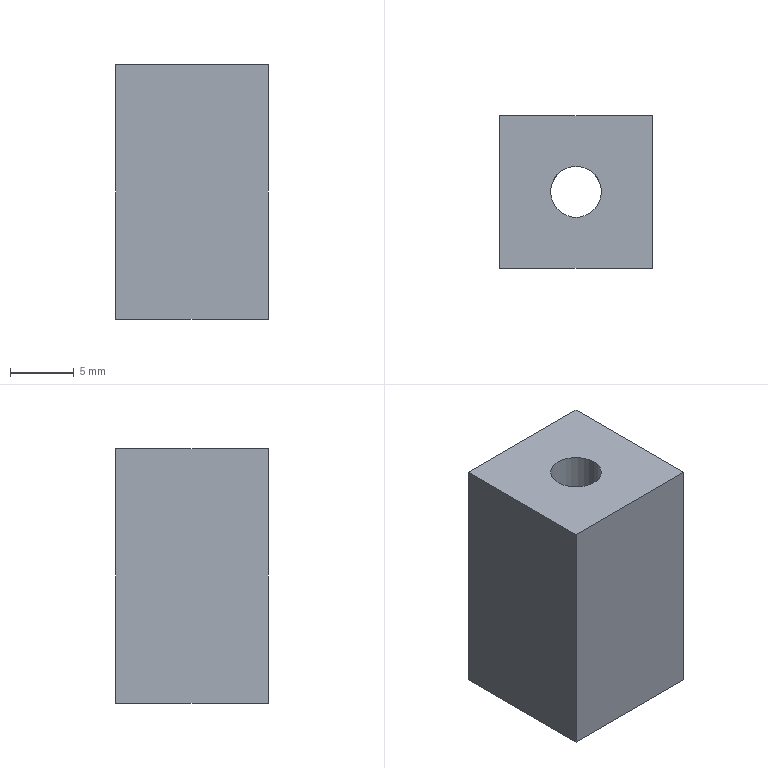Part | STEP file | Ngam kep 13 | 1 solid | 11 faces | box 12 x 12 x 20 mm | volume 2025 mm3 | plane 7 | cylinder 4 | commonest cylinder face diameters 4 x2 8 x2
STEP:
#1=CARTESIAN_POINT('',(0.,0.,0.));
#2=DIRECTION('',(0.,0.,1.));
#3=DIRECTION('',(1.,0.,0.));
#4=AXIS2_PLACEMENT_3D('',#1,#2,#3);
#5=CARTESIAN_POINT('',(-2.,0.,12.));
#6=VERTEX_POINT('',#5);
#7=CARTESIAN_POINT('',(-2.,0.,8.));
#8=VERTEX_POINT('',#7);
#9=CARTESIAN_POINT('',(-2.,0.,12.));
#10=DIRECTION('',(0.,0.,-1.));
#11=VECTOR('',#10,1.);
#12=LINE('',#9,#11);
#13=CARTESIAN_POINT('',(0.,0.,12.));
#14=DIRECTION('',(0.,0.,-1.));
#15=DIRECTION('',(-1.,0.,0.));
#16=AXIS2_PLACEMENT_3D('',#13,#14,#15);
#17=CYLINDRICAL_SURFACE('',#16,2.);
#18=CARTESIAN_POINT('',(6.283,0.));
#19=DIRECTION('',(0.,1.));
#20=VECTOR('',#19,1.);
#21=LINE('',#18,#20);
#22=(GEOMETRIC_REPRESENTATION_CONTEXT(2)PARAMETRIC_REPRESENTATION_CONTEXT()REPRESENTATION_CONTEXT('',''));
#23=DEFINITIONAL_REPRESENTATION('',(#21),#22);
#24=PCURVE('',#17,#23);
#25=CARTESIAN_POINT('',(0.,0.,12.));
#26=DIRECTION('',(0.,0.,-1.));
#27=DIRECTION('',(-1.,0.,0.));
#28=AXIS2_PLACEMENT_3D('',#25,#26,#27);
#29=CYLINDRICAL_SURFACE('',#28,2.);
#30=CARTESIAN_POINT('',(0.,0.));
#31=DIRECTION('',(0.,1.));
#32=VECTOR('',#31,1.);
#33=LINE('',#30,#32);
#34=(GEOMETRIC_REPRESENTATION_CONTEXT(2)PARAMETRIC_REPRESENTATION_CONTEXT()REPRESENTATION_CONTEXT('',''));
#35=DEFINITIONAL_REPRESENTATION('',(#33),#34);
#36=PCURVE('',#29,#35);
#37=SURFACE_CURVE('',#12,(#24,#36),.PCURVE_S1.);
#38=EDGE_CURVE('',#6,#8,#37,.T.);
#39=ORIENTED_EDGE('',*,*,#38,.T.);
#40=CARTESIAN_POINT('',(2.,0.,8.));
#41=VERTEX_POINT('',#40);
#42=CARTESIAN_POINT('',(0.,0.,8.));
#43=DIRECTION('',(0.,0.,1.));
#44=DIRECTION('',(1.,0.,0.));
#45=AXIS2_PLACEMENT_3D('',#42,#43,#44);
#46=CIRCLE('',#45,2.);
#47=CARTESIAN_POINT('',(9.425,4.));
#48=DIRECTION('',(-1.,0.));
#49=VECTOR('',#48,1.);
#50=LINE('',#47,#49);
#51=(GEOMETRIC_REPRESENTATION_CONTEXT(2)PARAMETRIC_REPRESENTATION_CONTEXT()REPRESENTATION_CONTEXT('',''));
#52=DEFINITIONAL_REPRESENTATION('',(#50),#51);
#53=PCURVE('',#17,#52);
#54=CARTESIAN_POINT('',(0.,0.,8.));
#55=DIRECTION('',(0.,0.,1.));
#56=DIRECTION('',(1.,0.,0.));
#57=AXIS2_PLACEMENT_3D('',#54,#55,#56);
#58=PLANE('',#57);
#59=CARTESIAN_POINT('',(0.,0.));
#60=DIRECTION('',(1.,0.));
#61=AXIS2_PLACEMENT_2D('',#59,#60);
#62=CIRCLE('',#61,2.);
#63=(GEOMETRIC_REPRESENTATION_CONTEXT(2)PARAMETRIC_REPRESENTATION_CONTEXT()REPRESENTATION_CONTEXT('',''));
#64=DEFINITIONAL_REPRESENTATION('',(#62),#63);
#65=PCURVE('',#58,#64);
#66=SURFACE_CURVE('',#46,(#53,#65),.PCURVE_S1.);
#67=EDGE_CURVE('',#8,#41,#66,.T.);
#68=ORIENTED_EDGE('',*,*,#67,.T.);
#69=CARTESIAN_POINT('',(2.,0.,12.));
#70=VERTEX_POINT('',#69);
#71=CARTESIAN_POINT('',(2.,0.,12.));
#72=DIRECTION('',(0.,0.,-1.));
#73=VECTOR('',#72,1.);
#74=LINE('',#71,#73);
#75=CARTESIAN_POINT('',(3.142,0.));
#76=DIRECTION('',(0.,1.));
#77=VECTOR('',#76,1.);
#78=LINE('',#75,#77);
#79=(GEOMETRIC_REPRESENTATION_CONTEXT(2)PARAMETRIC_REPRESENTATION_CONTEXT()REPRESENTATION_CONTEXT('',''));
#80=DEFINITIONAL_REPRESENTATION('',(#78),#79);
#81=PCURVE('',#17,#80);
#82=CARTESIAN_POINT('',(3.142,0.));
#83=DIRECTION('',(0.,1.));
#84=VECTOR('',#83,1.);
#85=LINE('',#82,#84);
#86=(GEOMETRIC_REPRESENTATION_CONTEXT(2)PARAMETRIC_REPRESENTATION_CONTEXT()REPRESENTATION_CONTEXT('',''));
#87=DEFINITIONAL_REPRESENTATION('',(#85),#86);
#88=PCURVE('',#29,#87);
#89=SURFACE_CURVE('',#74,(#81,#88),.PCURVE_S1.);
#90=EDGE_CURVE('',#70,#41,#89,.T.);
#91=ORIENTED_EDGE('',*,*,#90,.F.);
#92=CARTESIAN_POINT('',(0.,0.,12.));
#93=DIRECTION('',(0.,0.,1.));
#94=DIRECTION('',(1.,0.,0.));
#95=AXIS2_PLACEMENT_3D('',#92,#93,#94);
#96=CIRCLE('',#95,2.);
#97=CARTESIAN_POINT('',(9.425,0.));
#98=DIRECTION('',(-1.,0.));
#99=VECTOR('',#98,1.);
#100=LINE('',#97,#99);
#101=(GEOMETRIC_REPRESENTATION_CONTEXT(2)PARAMETRIC_REPRESENTATION_CONTEXT()REPRESENTATION_CONTEXT('',''));
#102=DEFINITIONAL_REPRESENTATION('',(#100),#101);
#103=PCURVE('',#17,#102);
#104=CARTESIAN_POINT('',(0.,0.,12.));
#105=DIRECTION('',(0.,0.,1.));
#106=DIRECTION('',(1.,0.,0.));
#107=AXIS2_PLACEMENT_3D('',#104,#105,#106);
#108=PLANE('',#107);
#109=CARTESIAN_POINT('',(0.,0.));
#110=DIRECTION('',(1.,0.));
#111=AXIS2_PLACEMENT_2D('',#109,#110);
#112=CIRCLE('',#111,2.);
#113=(GEOMETRIC_REPRESENTATION_CONTEXT(2)PARAMETRIC_REPRESENTATION_CONTEXT()REPRESENTATION_CONTEXT('',''));
#114=DEFINITIONAL_REPRESENTATION('',(#112),#113);
#115=PCURVE('',#108,#114);
#116=SURFACE_CURVE('',#96,(#103,#115),.PCURVE_S1.);
#117=EDGE_CURVE('',#6,#70,#116,.T.);
#118=ORIENTED_EDGE('',*,*,#117,.F.);
#119=EDGE_LOOP('',(#39,#68,#91,#118));
#120=FACE_BOUND('',#119,.F.);
#121=ADVANCED_FACE('',(#120),#17,.F.);
#122=CARTESIAN_POINT('',(-4.,0.,8.));
#123=VERTEX_POINT('',#122);
#124=CARTESIAN_POINT('',(-4.,0.,-8.));
#125=VERTEX_POINT('',#124);
#126=CARTESIAN_POINT('',(-4.,0.,8.));
#127=DIRECTION('',(0.,0.,-1.));
#128=VECTOR('',#127,1.);
#129=LINE('',#126,#128);
#130=CARTESIAN_POINT('',(0.,0.,8.));
#131=DIRECTION('',(0.,0.,-1.));
#132=DIRECTION('',(-1.,0.,0.));
#133=AXIS2_PLACEMENT_3D('',#130,#131,#132);
#134=CYLINDRICAL_SURFACE('',#133,4.);
#135=CARTESIAN_POINT('',(6.283,0.));
#136=DIRECTION('',(0.,1.));
#137=VECTOR('',#136,1.);
#138=LINE('',#135,#137);
#139=(GEOMETRIC_REPRESENTATION_CONTEXT(2)PARAMETRIC_REPRESENTATION_CONTEXT()REPRESENTATION_CONTEXT('',''));
#140=DEFINITIONAL_REPRESENTATION('',(#138),#139);
#141=PCURVE('',#134,#140);
#142=CARTESIAN_POINT('',(0.,0.,8.));
#143=DIRECTION('',(0.,0.,-1.));
#144=DIRECTION('',(-1.,0.,0.));
#145=AXIS2_PLACEMENT_3D('',#142,#143,#144);
#146=CYLINDRICAL_SURFACE('',#145,4.);
#147=CARTESIAN_POINT('',(0.,0.));
#148=DIRECTION('',(0.,1.));
#149=VECTOR('',#148,1.);
#150=LINE('',#147,#149);
#151=(GEOMETRIC_REPRESENTATION_CONTEXT(2)PARAMETRIC_REPRESENTATION_CONTEXT()REPRESENTATION_CONTEXT('',''));
#152=DEFINITIONAL_REPRESENTATION('',(#150),#151);
#153=PCURVE('',#146,#152);
#154=SURFACE_CURVE('',#129,(#141,#153),.PCURVE_S1.);
#155=EDGE_CURVE('',#123,#125,#154,.T.);
#156=ORIENTED_EDGE('',*,*,#155,.T.);
#157=CARTESIAN_POINT('',(4.,0.,-8.));
#158=VERTEX_POINT('',#157);
#159=CARTESIAN_POINT('',(0.,0.,-8.));
#160=DIRECTION('',(0.,0.,1.));
#161=DIRECTION('',(1.,0.,0.));
#162=AXIS2_PLACEMENT_3D('',#159,#160,#161);
#163=CIRCLE('',#162,4.);
#164=CARTESIAN_POINT('',(9.425,16.));
#165=DIRECTION('',(-1.,0.));
#166=VECTOR('',#165,1.);
#167=LINE('',#164,#166);
#168=(GEOMETRIC_REPRESENTATION_CONTEXT(2)PARAMETRIC_REPRESENTATION_CONTEXT()REPRESENTATION_CONTEXT('',''));
#169=DEFINITIONAL_REPRESENTATION('',(#167),#168);
#170=PCURVE('',#134,#169);
#171=CARTESIAN_POINT('',(0.,0.,-8.));
#172=DIRECTION('',(0.,0.,1.));
#173=DIRECTION('',(1.,0.,0.));
#174=AXIS2_PLACEMENT_3D('',#171,#172,#173);
#175=PLANE('',#174);
#176=CARTESIAN_POINT('',(0.,0.));
#177=DIRECTION('',(1.,0.));
#178=AXIS2_PLACEMENT_2D('',#176,#177);
#179=CIRCLE('',#178,4.);
#180=(GEOMETRIC_REPRESENTATION_CONTEXT(2)PARAMETRIC_REPRESENTATION_CONTEXT()REPRESENTATION_CONTEXT('',''));
#181=DEFINITIONAL_REPRESENTATION('',(#179),#180);
#182=PCURVE('',#175,#181);
#183=SURFACE_CURVE('',#163,(#170,#182),.PCURVE_S1.);
#184=EDGE_CURVE('',#125,#158,#183,.T.);
#185=ORIENTED_EDGE('',*,*,#184,.T.);
#186=CARTESIAN_POINT('',(4.,0.,8.));
#187=VERTEX_POINT('',#186);
#188=CARTESIAN_POINT('',(4.,0.,8.));
#189=DIRECTION('',(0.,0.,-1.));
#190=VECTOR('',#189,1.);
#191=LINE('',#188,#190);
#192=CARTESIAN_POINT('',(3.142,0.));
#193=DIRECTION('',(0.,1.));
#194=VECTOR('',#193,1.);
#195=LINE('',#192,#194);
#196=(GEOMETRIC_REPRESENTATION_CONTEXT(2)PARAMETRIC_REPRESENTATION_CONTEXT()REPRESENTATION_CONTEXT('',''));
#197=DEFINITIONAL_REPRESENTATION('',(#195),#196);
#198=PCURVE('',#134,#197);
#199=CARTESIAN_POINT('',(3.142,0.));
#200=DIRECTION('',(0.,1.));
#201=VECTOR('',#200,1.);
#202=LINE('',#199,#201);
#203=(GEOMETRIC_REPRESENTATION_CONTEXT(2)PARAMETRIC_REPRESENTATION_CONTEXT()REPRESENTATION_CONTEXT('',''));
#204=DEFINITIONAL_REPRESENTATION('',(#202),#203);
#205=PCURVE('',#146,#204);
#206=SURFACE_CURVE('',#191,(#198,#205),.PCURVE_S1.);
#207=EDGE_CURVE('',#187,#158,#206,.T.);
#208=ORIENTED_EDGE('',*,*,#207,.F.);
#209=CARTESIAN_POINT('',(0.,0.,8.));
#210=DIRECTION('',(0.,0.,1.));
#211=DIRECTION('',(1.,0.,0.));
#212=AXIS2_PLACEMENT_3D('',#209,#210,#211);
#213=CIRCLE('',#212,4.);
#214=CARTESIAN_POINT('',(9.425,0.));
#215=DIRECTION('',(-1.,0.));
#216=VECTOR('',#215,1.);
#217=LINE('',#214,#216);
#218=(GEOMETRIC_REPRESENTATION_CONTEXT(2)PARAMETRIC_REPRESENTATION_CONTEXT()REPRESENTATION_CONTEXT('',''));
#219=DEFINITIONAL_REPRESENTATION('',(#217),#218);
#220=PCURVE('',#134,#219);
#221=CARTESIAN_POINT('',(0.,0.));
#222=DIRECTION('',(1.,0.));
#223=AXIS2_PLACEMENT_2D('',#221,#222);
#224=CIRCLE('',#223,4.);
#225=(GEOMETRIC_REPRESENTATION_CONTEXT(2)PARAMETRIC_REPRESENTATION_CONTEXT()REPRESENTATION_CONTEXT('',''));
#226=DEFINITIONAL_REPRESENTATION('',(#224),#225);
#227=PCURVE('',#58,#226);
#228=SURFACE_CURVE('',#213,(#220,#227),.PCURVE_S1.);
#229=EDGE_CURVE('',#123,#187,#228,.T.);
#230=ORIENTED_EDGE('',*,*,#229,.F.);
#231=EDGE_LOOP('',(#156,#185,#208,#230));
#232=FACE_BOUND('',#231,.F.);
#233=ADVANCED_FACE('',(#232),#134,.F.);
#234=CARTESIAN_POINT('',(-6.,6.,-8.));
#235=VERTEX_POINT('',#234);
#236=CARTESIAN_POINT('',(-6.,-6.,-8.));
#237=VERTEX_POINT('',#236);
#238=CARTESIAN_POINT('',(-6.,6.,-8.));
#239=DIRECTION('',(0.,-1.,0.));
#240=VECTOR('',#239,1.);
#241=LINE('',#238,#240);
#242=CARTESIAN_POINT('',(-6.,6.));
#243=DIRECTION('',(0.,-1.));
#244=VECTOR('',#243,1.);
#245=LINE('',#242,#244);
#246=(GEOMETRIC_REPRESENTATION_CONTEXT(2)PARAMETRIC_REPRESENTATION_CONTEXT()REPRESENTATION_CONTEXT('',''));
#247=DEFINITIONAL_REPRESENTATION('',(#245),#246);
#248=PCURVE('',#175,#247);
#249=CARTESIAN_POINT('',(-6.,6.,8.));
#250=DIRECTION('',(1.,0.,0.));
#251=DIRECTION('',(0.,1.,0.));
#252=AXIS2_PLACEMENT_3D('',#249,#250,#251);
#253=PLANE('',#252);
#254=CARTESIAN_POINT('',(0.,-16.));
#255=DIRECTION('',(-1.,0.));
#256=VECTOR('',#255,1.);
#257=LINE('',#254,#256);
#258=(GEOMETRIC_REPRESENTATION_CONTEXT(2)PARAMETRIC_REPRESENTATION_CONTEXT()REPRESENTATION_CONTEXT('',''));
#259=DEFINITIONAL_REPRESENTATION('',(#257),#258);
#260=PCURVE('',#253,#259);
#261=SURFACE_CURVE('',#241,(#248,#260),.PCURVE_S1.);
#262=EDGE_CURVE('',#235,#237,#261,.T.);
#263=ORIENTED_EDGE('',*,*,#262,.F.);
#264=CARTESIAN_POINT('',(6.,6.,-8.));
#265=VERTEX_POINT('',#264);
#266=CARTESIAN_POINT('',(-6.,6.,-8.));
#267=DIRECTION('',(-1.,0.,0.));
#268=VECTOR('',#267,1.);
#269=LINE('',#266,#268);
#270=CARTESIAN_POINT('',(-6.,6.));
#271=DIRECTION('',(-1.,0.));
#272=VECTOR('',#271,1.);
#273=LINE('',#270,#272);
#274=(GEOMETRIC_REPRESENTATION_CONTEXT(2)PARAMETRIC_REPRESENTATION_CONTEXT()REPRESENTATION_CONTEXT('',''));
#275=DEFINITIONAL_REPRESENTATION('',(#273),#274);
#276=PCURVE('',#175,#275);
#277=CARTESIAN_POINT('',(-6.,6.,8.));
#278=DIRECTION('',(0.,-1.,0.));
#279=DIRECTION('',(0.,0.,-1.));
#280=AXIS2_PLACEMENT_3D('',#277,#278,#279);
#281=PLANE('',#280);
#282=CARTESIAN_POINT('',(16.,0.));
#283=DIRECTION('',(0.,-1.));
#284=VECTOR('',#283,1.);
#285=LINE('',#282,#284);
#286=(GEOMETRIC_REPRESENTATION_CONTEXT(2)PARAMETRIC_REPRESENTATION_CONTEXT()REPRESENTATION_CONTEXT('',''));
#287=DEFINITIONAL_REPRESENTATION('',(#285),#286);
#288=PCURVE('',#281,#287);
#289=SURFACE_CURVE('',#269,(#276,#288),.PCURVE_S1.);
#290=EDGE_CURVE('',#265,#235,#289,.T.);
#291=ORIENTED_EDGE('',*,*,#290,.F.);
#292=CARTESIAN_POINT('',(6.,-6.,-8.));
#293=VERTEX_POINT('',#292);
#294=CARTESIAN_POINT('',(6.,6.,-8.));
#295=DIRECTION('',(0.,1.,0.));
#296=VECTOR('',#295,1.);
#297=LINE('',#294,#296);
#298=CARTESIAN_POINT('',(6.,6.));
#299=DIRECTION('',(0.,1.));
#300=VECTOR('',#299,1.);
#301=LINE('',#298,#300);
#302=(GEOMETRIC_REPRESENTATION_CONTEXT(2)PARAMETRIC_REPRESENTATION_CONTEXT()REPRESENTATION_CONTEXT('',''));
#303=DEFINITIONAL_REPRESENTATION('',(#301),#302);
#304=PCURVE('',#175,#303);
#305=CARTESIAN_POINT('',(6.,6.,8.));
#306=DIRECTION('',(-1.,0.,0.));
#307=DIRECTION('',(0.,-1.,0.));
#308=AXIS2_PLACEMENT_3D('',#305,#306,#307);
#309=PLANE('',#308);
#310=CARTESIAN_POINT('',(0.,-16.));
#311=DIRECTION('',(-1.,0.));
#312=VECTOR('',#311,1.);
#313=LINE('',#310,#312);
#314=(GEOMETRIC_REPRESENTATION_CONTEXT(2)PARAMETRIC_REPRESENTATION_CONTEXT()REPRESENTATION_CONTEXT('',''));
#315=DEFINITIONAL_REPRESENTATION('',(#313),#314);
#316=PCURVE('',#309,#315);
#317=SURFACE_CURVE('',#297,(#304,#316),.PCURVE_S1.);
#318=EDGE_CURVE('',#293,#265,#317,.T.);
#319=ORIENTED_EDGE('',*,*,#318,.F.);
#320=CARTESIAN_POINT('',(-6.,-6.,-8.));
#321=DIRECTION('',(1.,0.,0.));
#322=VECTOR('',#321,1.);
#323=LINE('',#320,#322);
#324=CARTESIAN_POINT('',(-6.,-6.));
#325=DIRECTION('',(1.,0.));
#326=VECTOR('',#325,1.);
#327=LINE('',#324,#326);
#328=(GEOMETRIC_REPRESENTATION_CONTEXT(2)PARAMETRIC_REPRESENTATION_CONTEXT()REPRESENTATION_CONTEXT('',''));
#329=DEFINITIONAL_REPRESENTATION('',(#327),#328);
#330=PCURVE('',#175,#329);
#331=CARTESIAN_POINT('',(-6.,-6.,8.));
#332=DIRECTION('',(0.,1.,0.));
#333=DIRECTION('',(0.,0.,1.));
#334=AXIS2_PLACEMENT_3D('',#331,#332,#333);
#335=PLANE('',#334);
#336=CARTESIAN_POINT('',(-16.,0.));
#337=DIRECTION('',(0.,1.));
#338=VECTOR('',#337,1.);
#339=LINE('',#336,#338);
#340=(GEOMETRIC_REPRESENTATION_CONTEXT(2)PARAMETRIC_REPRESENTATION_CONTEXT()REPRESENTATION_CONTEXT('',''));
#341=DEFINITIONAL_REPRESENTATION('',(#339),#340);
#342=PCURVE('',#335,#341);
#343=SURFACE_CURVE('',#323,(#330,#342),.PCURVE_S1.);
#344=EDGE_CURVE('',#237,#293,#343,.T.);
#345=ORIENTED_EDGE('',*,*,#344,.F.);
#346=EDGE_LOOP('',(#263,#291,#319,#345));
#347=FACE_BOUND('',#346,.T.);
#348=ORIENTED_EDGE('',*,*,#184,.T.);
#349=CARTESIAN_POINT('',(0.,0.,-8.));
#350=DIRECTION('',(0.,0.,1.));
#351=DIRECTION('',(1.,0.,0.));
#352=AXIS2_PLACEMENT_3D('',#349,#350,#351);
#353=CIRCLE('',#352,4.);
#354=CARTESIAN_POINT('',(0.,0.));
#355=DIRECTION('',(1.,0.));
#356=AXIS2_PLACEMENT_2D('',#354,#355);
#357=CIRCLE('',#356,4.);
#358=(GEOMETRIC_REPRESENTATION_CONTEXT(2)PARAMETRIC_REPRESENTATION_CONTEXT()REPRESENTATION_CONTEXT('',''));
#359=DEFINITIONAL_REPRESENTATION('',(#357),#358);
#360=PCURVE('',#175,#359);
#361=CARTESIAN_POINT('',(3.142,16.));
#362=DIRECTION('',(-1.,0.));
#363=VECTOR('',#362,1.);
#364=LINE('',#361,#363);
#365=(GEOMETRIC_REPRESENTATION_CONTEXT(2)PARAMETRIC_REPRESENTATION_CONTEXT()REPRESENTATION_CONTEXT('',''));
#366=DEFINITIONAL_REPRESENTATION('',(#364),#365);
#367=PCURVE('',#146,#366);
#368=SURFACE_CURVE('',#353,(#360,#367),.PCURVE_S1.);
#369=EDGE_CURVE('',#158,#125,#368,.T.);
#370=ORIENTED_EDGE('',*,*,#369,.T.);
#371=EDGE_LOOP('',(#348,#370));
#372=FACE_BOUND('',#371,.T.);
#373=ADVANCED_FACE('',(#347,#372),#175,.F.);
#374=ORIENTED_EDGE('',*,*,#262,.T.);
#375=CARTESIAN_POINT('',(-6.,-6.,12.));
#376=VERTEX_POINT('',#375);
#377=CARTESIAN_POINT('',(-6.,-6.,8.));
#378=DIRECTION('',(0.,0.,-1.));
#379=VECTOR('',#378,1.);
#380=LINE('',#377,#379);
#381=CARTESIAN_POINT('',(-12.,0.));
#382=DIRECTION('',(0.,-1.));
#383=VECTOR('',#382,1.);
#384=LINE('',#381,#383);
#385=(GEOMETRIC_REPRESENTATION_CONTEXT(2)PARAMETRIC_REPRESENTATION_CONTEXT()REPRESENTATION_CONTEXT('',''));
#386=DEFINITIONAL_REPRESENTATION('',(#384),#385);
#387=PCURVE('',#253,#386);
#388=CARTESIAN_POINT('',(0.,0.));
#389=DIRECTION('',(-1.,0.));
#390=VECTOR('',#389,1.);
#391=LINE('',#388,#390);
#392=(GEOMETRIC_REPRESENTATION_CONTEXT(2)PARAMETRIC_REPRESENTATION_CONTEXT()REPRESENTATION_CONTEXT('',''));
#393=DEFINITIONAL_REPRESENTATION('',(#391),#392);
#394=PCURVE('',#335,#393);
#395=SURFACE_CURVE('',#380,(#387,#394),.PCURVE_S1.);
#396=EDGE_CURVE('',#376,#237,#395,.T.);
#397=ORIENTED_EDGE('',*,*,#396,.F.);
#398=CARTESIAN_POINT('',(-6.,6.,12.));
#399=VERTEX_POINT('',#398);
#400=CARTESIAN_POINT('',(-6.,6.,12.));
#401=DIRECTION('',(0.,-1.,0.));
#402=VECTOR('',#401,1.);
#403=LINE('',#400,#402);
#404=CARTESIAN_POINT('',(0.,4.));
#405=DIRECTION('',(-1.,0.));
#406=VECTOR('',#405,1.);
#407=LINE('',#404,#406);
#408=(GEOMETRIC_REPRESENTATION_CONTEXT(2)PARAMETRIC_REPRESENTATION_CONTEXT()REPRESENTATION_CONTEXT('',''));
#409=DEFINITIONAL_REPRESENTATION('',(#407),#408);
#410=PCURVE('',#253,#409);
#411=CARTESIAN_POINT('',(-6.,6.));
#412=DIRECTION('',(0.,-1.));
#413=VECTOR('',#412,1.);
#414=LINE('',#411,#413);
#415=(GEOMETRIC_REPRESENTATION_CONTEXT(2)PARAMETRIC_REPRESENTATION_CONTEXT()REPRESENTATION_CONTEXT('',''));
#416=DEFINITIONAL_REPRESENTATION('',(#414),#415);
#417=PCURVE('',#108,#416);
#418=SURFACE_CURVE('',#403,(#410,#417),.PCURVE_S1.);
#419=EDGE_CURVE('',#399,#376,#418,.T.);
#420=ORIENTED_EDGE('',*,*,#419,.F.);
#421=CARTESIAN_POINT('',(-6.,6.,8.));
#422=DIRECTION('',(0.,0.,-1.));
#423=VECTOR('',#422,1.);
#424=LINE('',#421,#423);
#425=CARTESIAN_POINT('',(0.,0.));
#426=DIRECTION('',(0.,-1.));
#427=VECTOR('',#426,1.);
#428=LINE('',#425,#427);
#429=(GEOMETRIC_REPRESENTATION_CONTEXT(2)PARAMETRIC_REPRESENTATION_CONTEXT()REPRESENTATION_CONTEXT('',''));
#430=DEFINITIONAL_REPRESENTATION('',(#428),#429);
#431=PCURVE('',#253,#430);
#432=CARTESIAN_POINT('',(0.,0.));
#433=DIRECTION('',(1.,0.));
#434=VECTOR('',#433,1.);
#435=LINE('',#432,#434);
#436=(GEOMETRIC_REPRESENTATION_CONTEXT(2)PARAMETRIC_REPRESENTATION_CONTEXT()REPRESENTATION_CONTEXT('',''));
#437=DEFINITIONAL_REPRESENTATION('',(#435),#436);
#438=PCURVE('',#281,#437);
#439=SURFACE_CURVE('',#424,(#431,#438),.PCURVE_S1.);
#440=EDGE_CURVE('',#399,#235,#439,.T.);
#441=ORIENTED_EDGE('',*,*,#440,.T.);
#442=EDGE_LOOP('',(#374,#397,#420,#441));
#443=FACE_BOUND('',#442,.T.);
#444=ADVANCED_FACE('',(#443),#253,.F.);
#445=ORIENTED_EDGE('',*,*,#344,.T.);
#446=CARTESIAN_POINT('',(6.,-6.,12.));
#447=VERTEX_POINT('',#446);
#448=CARTESIAN_POINT('',(6.,-6.,8.));
#449=DIRECTION('',(0.,0.,-1.));
#450=VECTOR('',#449,1.);
#451=LINE('',#448,#450);
#452=CARTESIAN_POINT('',(0.,12.));
#453=DIRECTION('',(-1.,0.));
#454=VECTOR('',#453,1.);
#455=LINE('',#452,#454);
#456=(GEOMETRIC_REPRESENTATION_CONTEXT(2)PARAMETRIC_REPRESENTATION_CONTEXT()REPRESENTATION_CONTEXT('',''));
#457=DEFINITIONAL_REPRESENTATION('',(#455),#456);
#458=PCURVE('',#335,#457);
#459=CARTESIAN_POINT('',(12.,0.));
#460=DIRECTION('',(0.,-1.));
#461=VECTOR('',#460,1.);
#462=LINE('',#459,#461);
#463=(GEOMETRIC_REPRESENTATION_CONTEXT(2)PARAMETRIC_REPRESENTATION_CONTEXT()REPRESENTATION_CONTEXT('',''));
#464=DEFINITIONAL_REPRESENTATION('',(#462),#463);
#465=PCURVE('',#309,#464);
#466=SURFACE_CURVE('',#451,(#458,#465),.PCURVE_S1.);
#467=EDGE_CURVE('',#447,#293,#466,.T.);
#468=ORIENTED_EDGE('',*,*,#467,.F.);
#469=CARTESIAN_POINT('',(-6.,-6.,12.));
#470=DIRECTION('',(1.,0.,0.));
#471=VECTOR('',#470,1.);
#472=LINE('',#469,#471);
#473=CARTESIAN_POINT('',(4.,0.));
#474=DIRECTION('',(0.,1.));
#475=VECTOR('',#474,1.);
#476=LINE('',#473,#475);
#477=(GEOMETRIC_REPRESENTATION_CONTEXT(2)PARAMETRIC_REPRESENTATION_CONTEXT()REPRESENTATION_CONTEXT('',''));
#478=DEFINITIONAL_REPRESENTATION('',(#476),#477);
#479=PCURVE('',#335,#478);
#480=CARTESIAN_POINT('',(-6.,-6.));
#481=DIRECTION('',(1.,0.));
#482=VECTOR('',#481,1.);
#483=LINE('',#480,#482);
#484=(GEOMETRIC_REPRESENTATION_CONTEXT(2)PARAMETRIC_REPRESENTATION_CONTEXT()REPRESENTATION_CONTEXT('',''));
#485=DEFINITIONAL_REPRESENTATION('',(#483),#484);
#486=PCURVE('',#108,#485);
#487=SURFACE_CURVE('',#472,(#479,#486),.PCURVE_S1.);
#488=EDGE_CURVE('',#376,#447,#487,.T.);
#489=ORIENTED_EDGE('',*,*,#488,.F.);
#490=ORIENTED_EDGE('',*,*,#396,.T.);
#491=EDGE_LOOP('',(#445,#468,#489,#490));
#492=FACE_BOUND('',#491,.T.);
#493=ADVANCED_FACE('',(#492),#335,.F.);
#494=ORIENTED_EDGE('',*,*,#318,.T.);
#495=CARTESIAN_POINT('',(6.,6.,12.));
#496=VERTEX_POINT('',#495);
#497=CARTESIAN_POINT('',(6.,6.,8.));
#498=DIRECTION('',(0.,0.,-1.));
#499=VECTOR('',#498,1.);
#500=LINE('',#497,#499);
#501=CARTESIAN_POINT('',(0.,0.));
#502=DIRECTION('',(0.,-1.));
#503=VECTOR('',#502,1.);
#504=LINE('',#501,#503);
#505=(GEOMETRIC_REPRESENTATION_CONTEXT(2)PARAMETRIC_REPRESENTATION_CONTEXT()REPRESENTATION_CONTEXT('',''));
#506=DEFINITIONAL_REPRESENTATION('',(#504),#505);
#507=PCURVE('',#309,#506);
#508=CARTESIAN_POINT('',(0.,12.));
#509=DIRECTION('',(1.,0.));
#510=VECTOR('',#509,1.);
#511=LINE('',#508,#510);
#512=(GEOMETRIC_REPRESENTATION_CONTEXT(2)PARAMETRIC_REPRESENTATION_CONTEXT()REPRESENTATION_CONTEXT('',''));
#513=DEFINITIONAL_REPRESENTATION('',(#511),#512);
#514=PCURVE('',#281,#513);
#515=SURFACE_CURVE('',#500,(#507,#514),.PCURVE_S1.);
#516=EDGE_CURVE('',#496,#265,#515,.T.);
#517=ORIENTED_EDGE('',*,*,#516,.F.);
#518=CARTESIAN_POINT('',(6.,-6.,12.));
#519=DIRECTION('',(0.,1.,0.));
#520=VECTOR('',#519,1.);
#521=LINE('',#518,#520);
#522=CARTESIAN_POINT('',(12.,4.));
#523=DIRECTION('',(-1.,0.));
#524=VECTOR('',#523,1.);
#525=LINE('',#522,#524);
#526=(GEOMETRIC_REPRESENTATION_CONTEXT(2)PARAMETRIC_REPRESENTATION_CONTEXT()REPRESENTATION_CONTEXT('',''));
#527=DEFINITIONAL_REPRESENTATION('',(#525),#526);
#528=PCURVE('',#309,#527);
#529=CARTESIAN_POINT('',(6.,-6.));
#530=DIRECTION('',(0.,1.));
#531=VECTOR('',#530,1.);
#532=LINE('',#529,#531);
#533=(GEOMETRIC_REPRESENTATION_CONTEXT(2)PARAMETRIC_REPRESENTATION_CONTEXT()REPRESENTATION_CONTEXT('',''));
#534=DEFINITIONAL_REPRESENTATION('',(#532),#533);
#535=PCURVE('',#108,#534);
#536=SURFACE_CURVE('',#521,(#528,#535),.PCURVE_S1.);
#537=EDGE_CURVE('',#447,#496,#536,.T.);
#538=ORIENTED_EDGE('',*,*,#537,.F.);
#539=ORIENTED_EDGE('',*,*,#467,.T.);
#540=EDGE_LOOP('',(#494,#517,#538,#539));
#541=FACE_BOUND('',#540,.T.);
#542=ADVANCED_FACE('',(#541),#309,.F.);
#543=ORIENTED_EDGE('',*,*,#290,.T.);
#544=ORIENTED_EDGE('',*,*,#440,.F.);
#545=CARTESIAN_POINT('',(6.,6.,12.));
#546=DIRECTION('',(-1.,0.,0.));
#547=VECTOR('',#546,1.);
#548=LINE('',#545,#547);
#549=CARTESIAN_POINT('',(-4.,12.));
#550=DIRECTION('',(0.,-1.));
#551=VECTOR('',#550,1.);
#552=LINE('',#549,#551);
#553=(GEOMETRIC_REPRESENTATION_CONTEXT(2)PARAMETRIC_REPRESENTATION_CONTEXT()REPRESENTATION_CONTEXT('',''));
#554=DEFINITIONAL_REPRESENTATION('',(#552),#553);
#555=PCURVE('',#281,#554);
#556=CARTESIAN_POINT('',(6.,6.));
#557=DIRECTION('',(-1.,0.));
#558=VECTOR('',#557,1.);
#559=LINE('',#556,#558);
#560=(GEOMETRIC_REPRESENTATION_CONTEXT(2)PARAMETRIC_REPRESENTATION_CONTEXT()REPRESENTATION_CONTEXT('',''));
#561=DEFINITIONAL_REPRESENTATION('',(#559),#560);
#562=PCURVE('',#108,#561);
#563=SURFACE_CURVE('',#548,(#555,#562),.PCURVE_S1.);
#564=EDGE_CURVE('',#496,#399,#563,.T.);
#565=ORIENTED_EDGE('',*,*,#564,.F.);
#566=ORIENTED_EDGE('',*,*,#516,.T.);
#567=EDGE_LOOP('',(#543,#544,#565,#566));
#568=FACE_BOUND('',#567,.T.);
#569=ADVANCED_FACE('',(#568),#281,.F.);
#570=ORIENTED_EDGE('',*,*,#369,.T.);
#571=ORIENTED_EDGE('',*,*,#155,.F.);
#572=CARTESIAN_POINT('',(0.,0.,8.));
#573=DIRECTION('',(0.,0.,1.));
#574=DIRECTION('',(1.,0.,0.));
#575=AXIS2_PLACEMENT_3D('',#572,#573,#574);
#576=CIRCLE('',#575,4.);
#577=CARTESIAN_POINT('',(3.142,0.));
#578=DIRECTION('',(-1.,0.));
#579=VECTOR('',#578,1.);
#580=LINE('',#577,#579);
#581=(GEOMETRIC_REPRESENTATION_CONTEXT(2)PARAMETRIC_REPRESENTATION_CONTEXT()REPRESENTATION_CONTEXT('',''));
#582=DEFINITIONAL_REPRESENTATION('',(#580),#581);
#583=PCURVE('',#146,#582);
#584=CARTESIAN_POINT('',(0.,0.));
#585=DIRECTION('',(1.,0.));
#586=AXIS2_PLACEMENT_2D('',#584,#585);
#587=CIRCLE('',#586,4.);
#588=(GEOMETRIC_REPRESENTATION_CONTEXT(2)PARAMETRIC_REPRESENTATION_CONTEXT()REPRESENTATION_CONTEXT('',''));
#589=DEFINITIONAL_REPRESENTATION('',(#587),#588);
#590=PCURVE('',#58,#589);
#591=SURFACE_CURVE('',#576,(#583,#590),.PCURVE_S1.);
#592=EDGE_CURVE('',#187,#123,#591,.T.);
#593=ORIENTED_EDGE('',*,*,#592,.F.);
#594=ORIENTED_EDGE('',*,*,#207,.T.);
#595=EDGE_LOOP('',(#570,#571,#593,#594));
#596=FACE_BOUND('',#595,.F.);
#597=ADVANCED_FACE('',(#596),#146,.F.);
#598=ORIENTED_EDGE('',*,*,#537,.T.);
#599=ORIENTED_EDGE('',*,*,#564,.T.);
#600=ORIENTED_EDGE('',*,*,#419,.T.);
#601=ORIENTED_EDGE('',*,*,#488,.T.);
#602=EDGE_LOOP('',(#598,#599,#600,#601));
#603=FACE_BOUND('',#602,.T.);
#604=ORIENTED_EDGE('',*,*,#117,.F.);
#605=CARTESIAN_POINT('',(0.,0.,12.));
#606=DIRECTION('',(0.,0.,1.));
#607=DIRECTION('',(1.,0.,0.));
#608=AXIS2_PLACEMENT_3D('',#605,#606,#607);
#609=CIRCLE('',#608,2.);
#610=CARTESIAN_POINT('',(0.,0.));
#611=DIRECTION('',(1.,0.));
#612=AXIS2_PLACEMENT_2D('',#610,#611);
#613=CIRCLE('',#612,2.);
#614=(GEOMETRIC_REPRESENTATION_CONTEXT(2)PARAMETRIC_REPRESENTATION_CONTEXT()REPRESENTATION_CONTEXT('',''));
#615=DEFINITIONAL_REPRESENTATION('',(#613),#614);
#616=PCURVE('',#108,#615);
#617=CARTESIAN_POINT('',(3.142,0.));
#618=DIRECTION('',(-1.,0.));
#619=VECTOR('',#618,1.);
#620=LINE('',#617,#619);
#621=(GEOMETRIC_REPRESENTATION_CONTEXT(2)PARAMETRIC_REPRESENTATION_CONTEXT()REPRESENTATION_CONTEXT('',''));
#622=DEFINITIONAL_REPRESENTATION('',(#620),#621);
#623=PCURVE('',#29,#622);
#624=SURFACE_CURVE('',#609,(#616,#623),.PCURVE_S1.);
#625=EDGE_CURVE('',#70,#6,#624,.T.);
#626=ORIENTED_EDGE('',*,*,#625,.F.);
#627=EDGE_LOOP('',(#604,#626));
#628=FACE_BOUND('',#627,.T.);
#629=ADVANCED_FACE('',(#603,#628),#108,.T.);
#630=ORIENTED_EDGE('',*,*,#229,.F.);
#631=ORIENTED_EDGE('',*,*,#592,.F.);
#632=EDGE_LOOP('',(#630,#631));
#633=FACE_BOUND('',#632,.T.);
#634=ORIENTED_EDGE('',*,*,#67,.T.);
#635=CARTESIAN_POINT('',(0.,0.,8.));
#636=DIRECTION('',(0.,0.,1.));
#637=DIRECTION('',(1.,0.,0.));
#638=AXIS2_PLACEMENT_3D('',#635,#636,#637);
#639=CIRCLE('',#638,2.);
#640=CARTESIAN_POINT('',(0.,0.));
#641=DIRECTION('',(1.,0.));
#642=AXIS2_PLACEMENT_2D('',#640,#641);
#643=CIRCLE('',#642,2.);
#644=(GEOMETRIC_REPRESENTATION_CONTEXT(2)PARAMETRIC_REPRESENTATION_CONTEXT()REPRESENTATION_CONTEXT('',''));
#645=DEFINITIONAL_REPRESENTATION('',(#643),#644);
#646=PCURVE('',#58,#645);
#647=CARTESIAN_POINT('',(3.142,4.));
#648=DIRECTION('',(-1.,0.));
#649=VECTOR('',#648,1.);
#650=LINE('',#647,#649);
#651=(GEOMETRIC_REPRESENTATION_CONTEXT(2)PARAMETRIC_REPRESENTATION_CONTEXT()REPRESENTATION_CONTEXT('',''));
#652=DEFINITIONAL_REPRESENTATION('',(#650),#651);
#653=PCURVE('',#29,#652);
#654=SURFACE_CURVE('',#639,(#646,#653),.PCURVE_S1.);
#655=EDGE_CURVE('',#41,#8,#654,.T.);
#656=ORIENTED_EDGE('',*,*,#655,.T.);
#657=EDGE_LOOP('',(#634,#656));
#658=FACE_BOUND('',#657,.T.);
#659=ADVANCED_FACE('',(#633,#658),#58,.F.);
#660=ORIENTED_EDGE('',*,*,#655,.T.);
#661=ORIENTED_EDGE('',*,*,#38,.F.);
#662=ORIENTED_EDGE('',*,*,#625,.F.);
#663=ORIENTED_EDGE('',*,*,#90,.T.);
#664=EDGE_LOOP('',(#660,#661,#662,#663));
#665=FACE_BOUND('',#664,.F.);
#666=ADVANCED_FACE('',(#665),#29,.F.);
#667=CLOSED_SHELL('',(#121,#233,#373,#444,#493,#542,#569,#597,#629,#659,#666));
#668=MANIFOLD_SOLID_BREP('',#667);
#669=(LENGTH_UNIT()NAMED_UNIT(*)SI_UNIT(.MILLI.,.METRE.));
#670=UNCERTAINTY_MEASURE_WITH_UNIT(LENGTH_MEASURE(0.0000001),#669,'','');
#671=(NAMED_UNIT(*)PLANE_ANGLE_UNIT()SI_UNIT($,.RADIAN.));
#672=(NAMED_UNIT(*)SI_UNIT($,.STERADIAN.)SOLID_ANGLE_UNIT());
#673=(GEOMETRIC_REPRESENTATION_CONTEXT(3)GLOBAL_UNCERTAINTY_ASSIGNED_CONTEXT((#670))GLOBAL_UNIT_ASSIGNED_CONTEXT((#669,#671,#672))REPRESENTATION_CONTEXT('',''));
#674=ADVANCED_BREP_SHAPE_REPRESENTATION('',(#4,#668),#673);